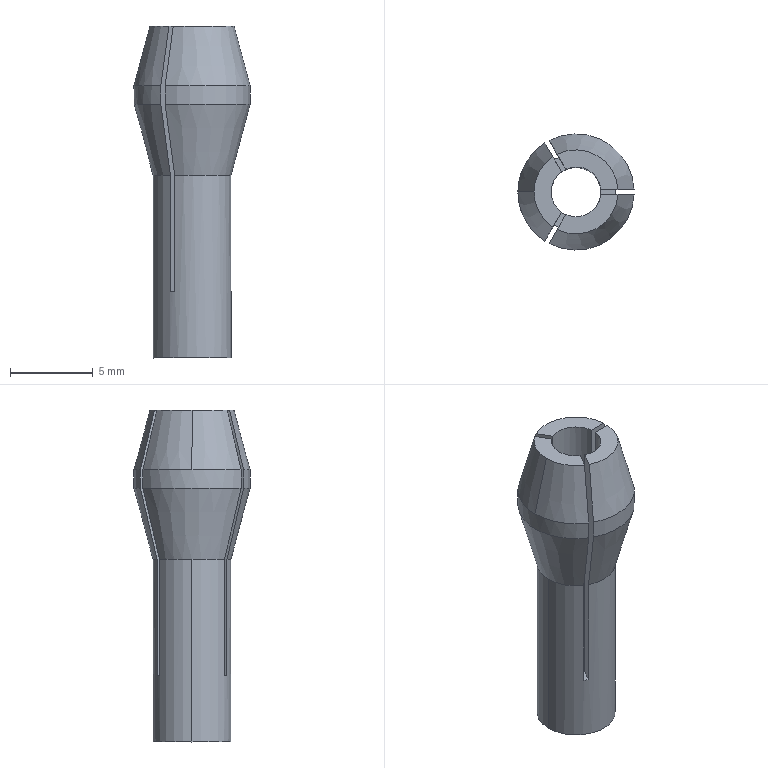Part | SolidWorks | features BaseBody 1 | 1 solid | 27 faces | box 6.997 x 7 x 20 mm | volume 294.902 mm3 | plane 13 | cylinder 7 | cone 7 | commonest cylinder face diameters 7 x3 3 x2 4.7 x2
STEP:
#1=CARTESIAN_POINT('',(482.037,37.715,102.045));
#2=VERTEX_POINT('',#1);
#3=CARTESIAN_POINT('',(479.037,37.715,102.045));
#4=VERTEX_POINT('',#3);
#5=CARTESIAN_POINT('',(480.537,37.715,102.045));
#6=DIRECTION('',(0.000000013,0.,-1.));
#7=DIRECTION('',(1.,0.,0.000000013));
#8=AXIS2_PLACEMENT_3D('',#5,#6,#7);
#9=CIRCLE('',#8,1.5);
#10=EDGE_CURVE('',#2,#4,#9,.T.);
#11=ORIENTED_EDGE('',*,*,#10,.T.);
#12=CARTESIAN_POINT('',(479.037,37.715,122.045));
#13=VERTEX_POINT('',#12);
#14=CARTESIAN_POINT('',(479.037,37.715,102.045));
#15=DIRECTION('',(-0.000000013,0.,1.));
#16=VECTOR('',#15,1000.);
#17=LINE('',#14,#16);
#18=EDGE_CURVE('',#4,#13,#17,.T.);
#19=ORIENTED_EDGE('',*,*,#18,.T.);
#20=CARTESIAN_POINT('',(479.661,36.497,122.045));
#21=VERTEX_POINT('',#20);
#22=CARTESIAN_POINT('',(480.537,37.715,122.045));
#23=DIRECTION('',(-0.000000013,0.,1.));
#24=DIRECTION('',(1.,0.,0.000000013));
#25=AXIS2_PLACEMENT_3D('',#22,#23,#24);
#26=CIRCLE('',#25,1.5);
#27=EDGE_CURVE('',#13,#21,#26,.T.);
#28=ORIENTED_EDGE('',*,*,#27,.T.);
#29=CARTESIAN_POINT('',(479.661,36.497,106.045));
#30=VERTEX_POINT('',#29);
#31=CARTESIAN_POINT('',(479.661,36.497,112.045));
#32=DIRECTION('',(0.000000013,0.,-1.));
#33=VECTOR('',#32,1000.);
#34=LINE('',#31,#33);
#35=EDGE_CURVE('',#21,#30,#34,.T.);
#36=ORIENTED_EDGE('',*,*,#35,.T.);
#37=CARTESIAN_POINT('',(479.921,36.347,106.045));
#38=VERTEX_POINT('',#37);
#39=CARTESIAN_POINT('',(480.537,37.715,106.045));
#40=DIRECTION('',(-0.000000013,0.,1.));
#41=DIRECTION('',(1.,0.,0.000000013));
#42=AXIS2_PLACEMENT_3D('',#39,#40,#41);
#43=CIRCLE('',#42,1.5);
#44=EDGE_CURVE('',#30,#38,#43,.T.);
#45=ORIENTED_EDGE('',*,*,#44,.T.);
#46=CARTESIAN_POINT('',(479.921,36.347,122.045));
#47=VERTEX_POINT('',#46);
#48=CARTESIAN_POINT('',(479.921,36.347,112.045));
#49=DIRECTION('',(-0.000000013,0.,1.));
#50=VECTOR('',#49,1000.);
#51=LINE('',#48,#50);
#52=EDGE_CURVE('',#38,#47,#51,.T.);
#53=ORIENTED_EDGE('',*,*,#52,.T.);
#54=CARTESIAN_POINT('',(482.029,37.565,122.045));
#55=VERTEX_POINT('',#54);
#56=CARTESIAN_POINT('',(480.537,37.715,122.045));
#57=DIRECTION('',(-0.000000013,0.,1.));
#58=DIRECTION('',(1.,0.,0.000000013));
#59=AXIS2_PLACEMENT_3D('',#56,#57,#58);
#60=CIRCLE('',#59,1.5);
#61=EDGE_CURVE('',#47,#55,#60,.T.);
#62=ORIENTED_EDGE('',*,*,#61,.T.);
#63=CARTESIAN_POINT('',(482.029,37.565,106.045));
#64=VERTEX_POINT('',#63);
#65=CARTESIAN_POINT('',(482.029,37.565,112.045));
#66=DIRECTION('',(0.000000013,0.,-1.));
#67=VECTOR('',#66,1000.);
#68=LINE('',#65,#67);
#69=EDGE_CURVE('',#55,#64,#68,.T.);
#70=ORIENTED_EDGE('',*,*,#69,.T.);
#71=CARTESIAN_POINT('',(482.037,37.715,106.045));
#72=VERTEX_POINT('',#71);
#73=CARTESIAN_POINT('',(480.537,37.715,106.045));
#74=DIRECTION('',(-0.000000013,0.,1.));
#75=DIRECTION('',(1.,0.,0.000000013));
#76=AXIS2_PLACEMENT_3D('',#73,#74,#75);
#77=CIRCLE('',#76,1.5);
#78=EDGE_CURVE('',#64,#72,#77,.T.);
#79=ORIENTED_EDGE('',*,*,#78,.T.);
#80=CARTESIAN_POINT('',(482.037,37.715,102.045));
#81=DIRECTION('',(-0.000000013,0.,1.));
#82=VECTOR('',#81,1000.);
#83=LINE('',#80,#82);
#84=EDGE_CURVE('',#2,#72,#83,.T.);
#85=ORIENTED_EDGE('',*,*,#84,.F.);
#86=EDGE_LOOP('',(#11,#19,#28,#36,#45,#53,#62,#70,#79,#85));
#87=FACE_OUTER_BOUND('',#86,.T.);
#88=CARTESIAN_POINT('',(480.537,37.715,102.045));
#89=DIRECTION('',(-0.000000013,0.,1.));
#90=DIRECTION('',(1.,0.,0.000000013));
#91=AXIS2_PLACEMENT_3D('',#88,#89,#90);
#92=CYLINDRICAL_SURFACE('',#91,1.5);
#93=ADVANCED_FACE('',(#87),#92,.F.);
#94=CARTESIAN_POINT('',(482.887,37.715,102.045));
#95=VERTEX_POINT('',#94);
#96=CARTESIAN_POINT('',(478.187,37.715,102.045));
#97=VERTEX_POINT('',#96);
#98=CARTESIAN_POINT('',(480.537,37.715,102.045));
#99=DIRECTION('',(-0.000000013,0.,1.));
#100=DIRECTION('',(1.,0.,0.000000013));
#101=AXIS2_PLACEMENT_3D('',#98,#99,#100);
#102=CIRCLE('',#101,2.35);
#103=EDGE_CURVE('',#95,#97,#102,.T.);
#104=ORIENTED_EDGE('',*,*,#103,.T.);
#105=CARTESIAN_POINT('',(478.187,37.715,113.045));
#106=VERTEX_POINT('',#105);
#107=CARTESIAN_POINT('',(478.187,37.715,102.045));
#108=DIRECTION('',(-0.000000013,0.,1.));
#109=VECTOR('',#108,1000.);
#110=LINE('',#107,#109);
#111=EDGE_CURVE('',#97,#106,#110,.T.);
#112=ORIENTED_EDGE('',*,*,#111,.T.);
#113=CARTESIAN_POINT('',(479.234,39.671,113.045));
#114=VERTEX_POINT('',#113);
#115=CARTESIAN_POINT('',(480.537,37.715,113.045));
#116=DIRECTION('',(-0.000000013,0.,1.));
#117=DIRECTION('',(0.,1.,0.));
#118=AXIS2_PLACEMENT_3D('',#115,#116,#117);
#119=CIRCLE('',#118,2.35);
#120=EDGE_CURVE('',#114,#106,#119,.T.);
#121=ORIENTED_EDGE('',*,*,#120,.F.);
#122=CARTESIAN_POINT('',(479.234,39.671,106.045));
#123=VERTEX_POINT('',#122);
#124=CARTESIAN_POINT('',(479.234,39.671,107.545));
#125=DIRECTION('',(-0.000000013,0.,1.));
#126=VECTOR('',#125,1000.);
#127=LINE('',#124,#126);
#128=EDGE_CURVE('',#123,#114,#127,.T.);
#129=ORIENTED_EDGE('',*,*,#128,.F.);
#130=CARTESIAN_POINT('',(479.494,39.821,106.045));
#131=VERTEX_POINT('',#130);
#132=CARTESIAN_POINT('',(480.537,37.715,106.045));
#133=DIRECTION('',(-0.000000013,0.,1.));
#134=DIRECTION('',(1.,0.,0.000000013));
#135=AXIS2_PLACEMENT_3D('',#132,#133,#134);
#136=CIRCLE('',#135,2.35);
#137=EDGE_CURVE('',#131,#123,#136,.T.);
#138=ORIENTED_EDGE('',*,*,#137,.F.);
#139=CARTESIAN_POINT('',(479.494,39.821,113.045));
#140=VERTEX_POINT('',#139);
#141=CARTESIAN_POINT('',(479.494,39.821,107.545));
#142=DIRECTION('',(0.000000013,0.,-1.));
#143=VECTOR('',#142,1000.);
#144=LINE('',#141,#143);
#145=EDGE_CURVE('',#140,#131,#144,.T.);
#146=ORIENTED_EDGE('',*,*,#145,.F.);
#147=CARTESIAN_POINT('',(482.882,37.865,113.045));
#148=VERTEX_POINT('',#147);
#149=CARTESIAN_POINT('',(480.537,37.715,113.045));
#150=DIRECTION('',(-0.000000013,0.,1.));
#151=DIRECTION('',(0.,1.,0.));
#152=AXIS2_PLACEMENT_3D('',#149,#150,#151);
#153=CIRCLE('',#152,2.35);
#154=EDGE_CURVE('',#148,#140,#153,.T.);
#155=ORIENTED_EDGE('',*,*,#154,.F.);
#156=CARTESIAN_POINT('',(482.882,37.865,106.045));
#157=VERTEX_POINT('',#156);
#158=CARTESIAN_POINT('',(482.882,37.865,114.045));
#159=DIRECTION('',(0.000000013,0.,-1.));
#160=VECTOR('',#159,1000.);
#161=LINE('',#158,#160);
#162=EDGE_CURVE('',#148,#157,#161,.T.);
#163=ORIENTED_EDGE('',*,*,#162,.T.);
#164=CARTESIAN_POINT('',(482.887,37.715,106.045));
#165=VERTEX_POINT('',#164);
#166=CARTESIAN_POINT('',(480.537,37.715,106.045));
#167=DIRECTION('',(-0.000000013,0.,1.));
#168=DIRECTION('',(1.,0.,0.000000013));
#169=AXIS2_PLACEMENT_3D('',#166,#167,#168);
#170=CIRCLE('',#169,2.35);
#171=EDGE_CURVE('',#165,#157,#170,.T.);
#172=ORIENTED_EDGE('',*,*,#171,.F.);
#173=CARTESIAN_POINT('',(482.887,37.715,102.045));
#174=DIRECTION('',(-0.000000013,0.,1.));
#175=VECTOR('',#174,1000.);
#176=LINE('',#173,#175);
#177=EDGE_CURVE('',#95,#165,#176,.T.);
#178=ORIENTED_EDGE('',*,*,#177,.F.);
#179=EDGE_LOOP('',(#104,#112,#121,#129,#138,#146,#155,#163,#172,#178));
#180=FACE_OUTER_BOUND('',#179,.T.);
#181=CARTESIAN_POINT('',(480.537,37.715,102.045));
#182=DIRECTION('',(-0.000000013,0.,1.));
#183=DIRECTION('',(1.,0.,0.000000013));
#184=AXIS2_PLACEMENT_3D('',#181,#182,#183);
#185=CYLINDRICAL_SURFACE('',#184,2.35);
#186=ADVANCED_FACE('',(#180),#185,.T.);
#187=CARTESIAN_POINT('',(478.004,37.715,122.045));
#188=VERTEX_POINT('',#187);
#189=CARTESIAN_POINT('',(479.143,35.6,122.045));
#190=VERTEX_POINT('',#189);
#191=CARTESIAN_POINT('',(480.537,37.715,122.045));
#192=DIRECTION('',(-0.000000013,0.,1.));
#193=DIRECTION('',(-1.,0.,-0.000000013));
#194=AXIS2_PLACEMENT_3D('',#191,#192,#193);
#195=CIRCLE('',#194,2.533);
#196=EDGE_CURVE('',#188,#190,#195,.T.);
#197=ORIENTED_EDGE('',*,*,#196,.F.);
#198=CARTESIAN_POINT('',(477.037,37.715,118.437));
#199=VERTEX_POINT('',#198);
#200=CARTESIAN_POINT('',(477.037,37.715,118.437));
#201=DIRECTION('',(-0.2588,0.,-0.9659));
#202=VECTOR('',#201,1000.);
#203=LINE('',#200,#202);
#204=EDGE_CURVE('',#188,#199,#203,.T.);
#205=ORIENTED_EDGE('',*,*,#204,.T.);
#206=CARTESIAN_POINT('',(478.659,34.761,118.437));
#207=VERTEX_POINT('',#206);
#208=CARTESIAN_POINT('',(480.537,37.715,118.437));
#209=DIRECTION('',(0.000000013,0.,-1.));
#210=DIRECTION('',(0.,1.,0.));
#211=AXIS2_PLACEMENT_3D('',#208,#209,#210);
#212=CIRCLE('',#211,3.5);
#213=EDGE_CURVE('',#207,#199,#212,.T.);
#214=ORIENTED_EDGE('',*,*,#213,.F.);
#215=CARTESIAN_POINT('',(478.659,34.761,118.437));
#216=CARTESIAN_POINT('',(478.82,35.041,119.64));
#217=CARTESIAN_POINT('',(478.981,35.32,120.842));
#218=CARTESIAN_POINT('',(479.143,35.6,122.045));
#219=B_SPLINE_CURVE_WITH_KNOTS('',3,(#215,#216,#217,#218),.UNSPECIFIED.,.F.,.F.,(4,4),(0.,0.003736),.UNSPECIFIED.);
#220=EDGE_CURVE('',#207,#190,#219,.T.);
#221=ORIENTED_EDGE('',*,*,#220,.T.);
#222=EDGE_LOOP('',(#197,#205,#214,#221));
#223=FACE_OUTER_BOUND('',#222,.T.);
#224=CARTESIAN_POINT('',(480.537,37.715,118.437));
#225=DIRECTION('',(0.000000013,0.,-1.));
#226=DIRECTION('',(-1.,0.,-0.000000013));
#227=AXIS2_PLACEMENT_3D('',#224,#225,#226);
#228=CONICAL_SURFACE('',#227,3.5,0.2618);
#229=ADVANCED_FACE('',(#223),#228,.T.);
#230=ORIENTED_EDGE('',*,*,#18,.F.);
#231=CARTESIAN_POINT('',(480.537,37.715,102.045));
#232=DIRECTION('',(0.000000013,0.,-1.));
#233=DIRECTION('',(1.,0.,0.000000013));
#234=AXIS2_PLACEMENT_3D('',#231,#232,#233);
#235=CIRCLE('',#234,1.5);
#236=EDGE_CURVE('',#4,#2,#235,.T.);
#237=ORIENTED_EDGE('',*,*,#236,.T.);
#238=ORIENTED_EDGE('',*,*,#84,.T.);
#239=CARTESIAN_POINT('',(482.029,37.865,106.045));
#240=VERTEX_POINT('',#239);
#241=CARTESIAN_POINT('',(480.537,37.715,106.045));
#242=DIRECTION('',(-0.000000013,0.,1.));
#243=DIRECTION('',(1.,0.,0.000000013));
#244=AXIS2_PLACEMENT_3D('',#241,#242,#243);
#245=CIRCLE('',#244,1.5);
#246=EDGE_CURVE('',#72,#240,#245,.T.);
#247=ORIENTED_EDGE('',*,*,#246,.T.);
#248=CARTESIAN_POINT('',(482.029,37.865,122.045));
#249=VERTEX_POINT('',#248);
#250=CARTESIAN_POINT('',(482.029,37.865,112.045));
#251=DIRECTION('',(-0.000000013,0.,1.));
#252=VECTOR('',#251,1000.);
#253=LINE('',#250,#252);
#254=EDGE_CURVE('',#240,#249,#253,.T.);
#255=ORIENTED_EDGE('',*,*,#254,.T.);
#256=CARTESIAN_POINT('',(479.921,39.082,122.045));
#257=VERTEX_POINT('',#256);
#258=CARTESIAN_POINT('',(480.537,37.715,122.045));
#259=DIRECTION('',(-0.000000013,0.,1.));
#260=DIRECTION('',(1.,0.,0.000000013));
#261=AXIS2_PLACEMENT_3D('',#258,#259,#260);
#262=CIRCLE('',#261,1.5);
#263=EDGE_CURVE('',#249,#257,#262,.T.);
#264=ORIENTED_EDGE('',*,*,#263,.T.);
#265=CARTESIAN_POINT('',(479.921,39.082,106.045));
#266=VERTEX_POINT('',#265);
#267=CARTESIAN_POINT('',(479.921,39.082,112.045));
#268=DIRECTION('',(0.000000013,0.,-1.));
#269=VECTOR('',#268,1000.);
#270=LINE('',#267,#269);
#271=EDGE_CURVE('',#257,#266,#270,.T.);
#272=ORIENTED_EDGE('',*,*,#271,.T.);
#273=CARTESIAN_POINT('',(479.661,38.932,106.045));
#274=VERTEX_POINT('',#273);
#275=CARTESIAN_POINT('',(480.537,37.715,106.045));
#276=DIRECTION('',(-0.000000013,0.,1.));
#277=DIRECTION('',(1.,0.,0.000000013));
#278=AXIS2_PLACEMENT_3D('',#275,#276,#277);
#279=CIRCLE('',#278,1.5);
#280=EDGE_CURVE('',#266,#274,#279,.T.);
#281=ORIENTED_EDGE('',*,*,#280,.T.);
#282=CARTESIAN_POINT('',(479.661,38.932,122.045));
#283=VERTEX_POINT('',#282);
#284=CARTESIAN_POINT('',(479.661,38.932,112.045));
#285=DIRECTION('',(-0.000000013,0.,1.));
#286=VECTOR('',#285,1000.);
#287=LINE('',#284,#286);
#288=EDGE_CURVE('',#274,#283,#287,.T.);
#289=ORIENTED_EDGE('',*,*,#288,.T.);
#290=CARTESIAN_POINT('',(480.537,37.715,122.045));
#291=DIRECTION('',(-0.000000013,0.,1.));
#292=DIRECTION('',(1.,0.,0.000000013));
#293=AXIS2_PLACEMENT_3D('',#290,#291,#292);
#294=CIRCLE('',#293,1.5);
#295=EDGE_CURVE('',#283,#13,#294,.T.);
#296=ORIENTED_EDGE('',*,*,#295,.T.);
#297=EDGE_LOOP('',(#230,#237,#238,#247,#255,#264,#272,#281,#289,#296));
#298=FACE_OUTER_BOUND('',#297,.T.);
#299=CARTESIAN_POINT('',(480.537,37.715,102.045));
#300=DIRECTION('',(-0.000000013,0.,1.));
#301=DIRECTION('',(1.,0.,0.000000013));
#302=AXIS2_PLACEMENT_3D('',#299,#300,#301);
#303=CYLINDRICAL_SURFACE('',#302,1.5);
#304=ADVANCED_FACE('',(#298),#303,.F.);
#305=ORIENTED_EDGE('',*,*,#10,.F.);
#306=ORIENTED_EDGE('',*,*,#236,.F.);
#307=EDGE_LOOP('',(#305,#306));
#308=FACE_BOUND('',#307,.T.);
#309=ORIENTED_EDGE('',*,*,#103,.F.);
#310=CARTESIAN_POINT('',(480.537,37.715,102.045));
#311=DIRECTION('',(-0.000000013,0.,1.));
#312=DIRECTION('',(1.,0.,0.000000013));
#313=AXIS2_PLACEMENT_3D('',#310,#311,#312);
#314=CIRCLE('',#313,2.35);
#315=EDGE_CURVE('',#97,#95,#314,.T.);
#316=ORIENTED_EDGE('',*,*,#315,.F.);
#317=EDGE_LOOP('',(#309,#316));
#318=FACE_OUTER_BOUND('',#317,.T.);
#319=CARTESIAN_POINT('',(482.981,35.271,102.045));
#320=DIRECTION('',(-0.000000013,0.,1.));
#321=DIRECTION('',(0.,1.,0.));
#322=AXIS2_PLACEMENT_3D('',#319,#320,#321);
#323=PLANE('',#322);
#324=ADVANCED_FACE('',(#308,#318),#323,.F.);
#325=CARTESIAN_POINT('',(483.066,37.865,122.045));
#326=VERTEX_POINT('',#325);
#327=CARTESIAN_POINT('',(479.402,39.98,122.045));
#328=VERTEX_POINT('',#327);
#329=CARTESIAN_POINT('',(480.537,37.715,122.045));
#330=DIRECTION('',(-0.000000013,0.,1.));
#331=DIRECTION('',(-1.,0.,-0.000000013));
#332=AXIS2_PLACEMENT_3D('',#329,#330,#331);
#333=CIRCLE('',#332,2.533);
#334=EDGE_CURVE('',#326,#328,#333,.T.);
#335=ORIENTED_EDGE('',*,*,#334,.T.);
#336=CARTESIAN_POINT('',(479.402,39.98,122.045));
#337=DIRECTION('',(0.5,-0.866,0.000000006));
#338=VECTOR('',#337,1000.);
#339=LINE('',#336,#338);
#340=EDGE_CURVE('',#328,#257,#339,.T.);
#341=ORIENTED_EDGE('',*,*,#340,.T.);
#342=ORIENTED_EDGE('',*,*,#263,.F.);
#343=CARTESIAN_POINT('',(480.535,37.865,122.045));
#344=DIRECTION('',(1.,0.,0.000000013));
#345=VECTOR('',#344,1000.);
#346=LINE('',#343,#345);
#347=EDGE_CURVE('',#249,#326,#346,.T.);
#348=ORIENTED_EDGE('',*,*,#347,.T.);
#349=EDGE_LOOP('',(#335,#341,#342,#348));
#350=FACE_OUTER_BOUND('',#349,.T.);
#351=CARTESIAN_POINT('',(483.167,35.078,122.045));
#352=DIRECTION('',(-0.000000013,0.,1.));
#353=DIRECTION('',(0.,1.,0.));
#354=AXIS2_PLACEMENT_3D('',#351,#352,#353);
#355=PLANE('',#354);
#356=ADVANCED_FACE('',(#350),#355,.T.);
#357=ORIENTED_EDGE('',*,*,#254,.F.);
#358=CARTESIAN_POINT('',(483.031,37.865,106.045));
#359=DIRECTION('',(-1.,0.,-0.000000013));
#360=VECTOR('',#359,1000.);
#361=LINE('',#358,#360);
#362=EDGE_CURVE('',#157,#240,#361,.T.);
#363=ORIENTED_EDGE('',*,*,#362,.F.);
#364=ORIENTED_EDGE('',*,*,#162,.F.);
#365=CARTESIAN_POINT('',(484.034,37.865,117.337));
#366=VERTEX_POINT('',#365);
#367=CARTESIAN_POINT('',(484.034,37.865,117.337));
#368=CARTESIAN_POINT('',(483.65,37.865,115.906));
#369=CARTESIAN_POINT('',(483.266,37.865,114.476));
#370=CARTESIAN_POINT('',(482.882,37.865,113.045));
#371=B_SPLINE_CURVE_WITH_KNOTS('',3,(#367,#368,#369,#370),.UNSPECIFIED.,.F.,.F.,(4,4),(0.,0.004444),.UNSPECIFIED.);
#372=EDGE_CURVE('',#366,#148,#371,.T.);
#373=ORIENTED_EDGE('',*,*,#372,.F.);
#374=CARTESIAN_POINT('',(484.034,37.865,118.437));
#375=VERTEX_POINT('',#374);
#376=CARTESIAN_POINT('',(484.034,37.865,117.887));
#377=DIRECTION('',(-0.000000013,0.,1.));
#378=VECTOR('',#377,1000.);
#379=LINE('',#376,#378);
#380=EDGE_CURVE('',#366,#375,#379,.T.);
#381=ORIENTED_EDGE('',*,*,#380,.T.);
#382=CARTESIAN_POINT('',(483.066,37.865,122.045));
#383=CARTESIAN_POINT('',(483.388,37.865,120.842));
#384=CARTESIAN_POINT('',(483.711,37.865,119.64));
#385=CARTESIAN_POINT('',(484.034,37.865,118.437));
#386=B_SPLINE_CURVE_WITH_KNOTS('',3,(#382,#383,#384,#385),.UNSPECIFIED.,.F.,.F.,(4,4),(0.,0.003736),.UNSPECIFIED.);
#387=EDGE_CURVE('',#326,#375,#386,.T.);
#388=ORIENTED_EDGE('',*,*,#387,.F.);
#389=ORIENTED_EDGE('',*,*,#347,.F.);
#390=EDGE_LOOP('',(#357,#363,#364,#373,#381,#388,#389));
#391=FACE_OUTER_BOUND('',#390,.T.);
#392=CARTESIAN_POINT('',(484.074,37.865,105.725));
#393=DIRECTION('',(0.,1.,0.));
#394=DIRECTION('',(-1.,0.,-0.000000013));
#395=AXIS2_PLACEMENT_3D('',#392,#393,#394);
#396=PLANE('',#395);
#397=ADVANCED_FACE('',(#391),#396,.F.);
#398=ORIENTED_EDGE('',*,*,#78,.F.);
#399=CARTESIAN_POINT('',(482.882,37.565,106.045));
#400=VERTEX_POINT('',#399);
#401=CARTESIAN_POINT('',(482.458,37.565,106.045));
#402=DIRECTION('',(1.,0.,0.000000013));
#403=VECTOR('',#402,1000.);
#404=LINE('',#401,#403);
#405=EDGE_CURVE('',#64,#400,#404,.T.);
#406=ORIENTED_EDGE('',*,*,#405,.T.);
#407=CARTESIAN_POINT('',(480.537,37.715,106.045));
#408=DIRECTION('',(-0.000000013,0.,1.));
#409=DIRECTION('',(1.,0.,0.000000013));
#410=AXIS2_PLACEMENT_3D('',#407,#408,#409);
#411=CIRCLE('',#410,2.35);
#412=EDGE_CURVE('',#400,#165,#411,.T.);
#413=ORIENTED_EDGE('',*,*,#412,.T.);
#414=ORIENTED_EDGE('',*,*,#171,.T.);
#415=ORIENTED_EDGE('',*,*,#362,.T.);
#416=ORIENTED_EDGE('',*,*,#246,.F.);
#417=EDGE_LOOP('',(#398,#406,#413,#414,#415,#416));
#418=FACE_OUTER_BOUND('',#417,.T.);
#419=CARTESIAN_POINT('',(482.003,37.891,106.045));
#420=DIRECTION('',(-0.000000013,0.,1.));
#421=DIRECTION('',(0.,-1.,0.));
#422=AXIS2_PLACEMENT_3D('',#419,#420,#421);
#423=PLANE('',#422);
#424=ADVANCED_FACE('',(#418),#423,.T.);
#425=CARTESIAN_POINT('',(484.034,37.565,118.437));
#426=VERTEX_POINT('',#425);
#427=CARTESIAN_POINT('',(483.066,37.565,122.045));
#428=VERTEX_POINT('',#427);
#429=CARTESIAN_POINT('',(484.034,37.565,118.437));
#430=CARTESIAN_POINT('',(483.711,37.565,119.64));
#431=CARTESIAN_POINT('',(483.388,37.565,120.842));
#432=CARTESIAN_POINT('',(483.066,37.565,122.045));
#433=B_SPLINE_CURVE_WITH_KNOTS('',3,(#429,#430,#431,#432),.UNSPECIFIED.,.F.,.F.,(4,4),(0.,0.003736),.UNSPECIFIED.);
#434=EDGE_CURVE('',#426,#428,#433,.T.);
#435=ORIENTED_EDGE('',*,*,#434,.F.);
#436=CARTESIAN_POINT('',(484.034,37.565,117.337));
#437=VERTEX_POINT('',#436);
#438=CARTESIAN_POINT('',(484.034,37.565,117.887));
#439=DIRECTION('',(0.000000013,0.,-1.));
#440=VECTOR('',#439,1000.);
#441=LINE('',#438,#440);
#442=EDGE_CURVE('',#426,#437,#441,.T.);
#443=ORIENTED_EDGE('',*,*,#442,.T.);
#444=CARTESIAN_POINT('',(482.882,37.565,113.045));
#445=VERTEX_POINT('',#444);
#446=CARTESIAN_POINT('',(482.882,37.565,113.045));
#447=CARTESIAN_POINT('',(483.205,37.565,114.247));
#448=CARTESIAN_POINT('',(483.527,37.565,115.449));
#449=CARTESIAN_POINT('',(483.85,37.565,116.651));
#450=CARTESIAN_POINT('',(483.911,37.565,116.88));
#451=CARTESIAN_POINT('',(483.972,37.565,117.108));
#452=CARTESIAN_POINT('',(484.034,37.565,117.337));
#453=B_SPLINE_CURVE_WITH_KNOTS('',3,(#446,#447,#448,#449,#450,#451,#452),.UNSPECIFIED.,.F.,.F.,(4,3,4),(0.,0.003734,0.004444),.UNSPECIFIED.);
#454=EDGE_CURVE('',#445,#437,#453,.T.);
#455=ORIENTED_EDGE('',*,*,#454,.F.);
#456=CARTESIAN_POINT('',(482.882,37.565,114.045));
#457=DIRECTION('',(-0.000000013,0.,1.));
#458=VECTOR('',#457,1000.);
#459=LINE('',#456,#458);
#460=EDGE_CURVE('',#400,#445,#459,.T.);
#461=ORIENTED_EDGE('',*,*,#460,.F.);
#462=ORIENTED_EDGE('',*,*,#405,.F.);
#463=ORIENTED_EDGE('',*,*,#69,.F.);
#464=CARTESIAN_POINT('',(483.031,37.565,122.045));
#465=DIRECTION('',(-1.,0.,-0.000000013));
#466=VECTOR('',#465,1000.);
#467=LINE('',#464,#466);
#468=EDGE_CURVE('',#428,#55,#467,.T.);
#469=ORIENTED_EDGE('',*,*,#468,.F.);
#470=EDGE_LOOP('',(#435,#443,#455,#461,#462,#463,#469));
#471=FACE_OUTER_BOUND('',#470,.T.);
#472=CARTESIAN_POINT('',(481.989,37.565,105.725));
#473=DIRECTION('',(0.,-1.,0.));
#474=DIRECTION('',(1.,0.,0.000000013));
#475=AXIS2_PLACEMENT_3D('',#472,#473,#474);
#476=PLANE('',#475);
#477=ADVANCED_FACE('',(#471),#476,.F.);
#478=ORIENTED_EDGE('',*,*,#61,.F.);
#479=CARTESIAN_POINT('',(479.402,35.45,122.045));
#480=VERTEX_POINT('',#479);
#481=CARTESIAN_POINT('',(479.921,36.347,122.045));
#482=DIRECTION('',(-0.5,-0.866,-0.000000006));
#483=VECTOR('',#482,1000.);
#484=LINE('',#481,#483);
#485=EDGE_CURVE('',#47,#480,#484,.T.);
#486=ORIENTED_EDGE('',*,*,#485,.T.);
#487=CARTESIAN_POINT('',(480.537,37.715,122.045));
#488=DIRECTION('',(-0.000000013,0.,1.));
#489=DIRECTION('',(-1.,0.,-0.000000013));
#490=AXIS2_PLACEMENT_3D('',#487,#488,#489);
#491=CIRCLE('',#490,2.533);
#492=EDGE_CURVE('',#480,#428,#491,.T.);
#493=ORIENTED_EDGE('',*,*,#492,.T.);
#494=ORIENTED_EDGE('',*,*,#468,.T.);
#495=EDGE_LOOP('',(#478,#486,#493,#494));
#496=FACE_OUTER_BOUND('',#495,.T.);
#497=CARTESIAN_POINT('',(483.167,35.078,122.045));
#498=DIRECTION('',(-0.000000013,0.,1.));
#499=DIRECTION('',(0.,1.,0.));
#500=AXIS2_PLACEMENT_3D('',#497,#498,#499);
#501=PLANE('',#500);
#502=ADVANCED_FACE('',(#496),#501,.T.);
#503=ORIENTED_EDGE('',*,*,#111,.F.);
#504=ORIENTED_EDGE('',*,*,#315,.T.);
#505=ORIENTED_EDGE('',*,*,#177,.T.);
#506=ORIENTED_EDGE('',*,*,#412,.F.);
#507=ORIENTED_EDGE('',*,*,#460,.T.);
#508=CARTESIAN_POINT('',(479.494,35.609,113.045));
#509=VERTEX_POINT('',#508);
#510=CARTESIAN_POINT('',(480.537,37.715,113.045));
#511=DIRECTION('',(-0.000000013,0.,1.));
#512=DIRECTION('',(0.,1.,0.));
#513=AXIS2_PLACEMENT_3D('',#510,#511,#512);
#514=CIRCLE('',#513,2.35);
#515=EDGE_CURVE('',#509,#445,#514,.T.);
#516=ORIENTED_EDGE('',*,*,#515,.F.);
#517=CARTESIAN_POINT('',(479.494,35.609,106.045));
#518=VERTEX_POINT('',#517);
#519=CARTESIAN_POINT('',(479.494,35.609,107.545));
#520=DIRECTION('',(-0.000000013,0.,1.));
#521=VECTOR('',#520,1000.);
#522=LINE('',#519,#521);
#523=EDGE_CURVE('',#518,#509,#522,.T.);
#524=ORIENTED_EDGE('',*,*,#523,.F.);
#525=CARTESIAN_POINT('',(479.234,35.759,106.045));
#526=VERTEX_POINT('',#525);
#527=CARTESIAN_POINT('',(480.537,37.715,106.045));
#528=DIRECTION('',(-0.000000013,0.,1.));
#529=DIRECTION('',(1.,0.,0.000000013));
#530=AXIS2_PLACEMENT_3D('',#527,#528,#529);
#531=CIRCLE('',#530,2.35);
#532=EDGE_CURVE('',#526,#518,#531,.T.);
#533=ORIENTED_EDGE('',*,*,#532,.F.);
#534=CARTESIAN_POINT('',(479.234,35.759,113.045));
#535=VERTEX_POINT('',#534);
#536=CARTESIAN_POINT('',(479.234,35.759,107.545));
#537=DIRECTION('',(0.000000013,0.,-1.));
#538=VECTOR('',#537,1000.);
#539=LINE('',#536,#538);
#540=EDGE_CURVE('',#535,#526,#539,.T.);
#541=ORIENTED_EDGE('',*,*,#540,.F.);
#542=CARTESIAN_POINT('',(480.537,37.715,113.045));
#543=DIRECTION('',(-0.000000013,0.,1.));
#544=DIRECTION('',(0.,1.,0.));
#545=AXIS2_PLACEMENT_3D('',#542,#543,#544);
#546=CIRCLE('',#545,2.35);
#547=EDGE_CURVE('',#106,#535,#546,.T.);
#548=ORIENTED_EDGE('',*,*,#547,.F.);
#549=EDGE_LOOP('',(#503,#504,#505,#506,#507,#516,#524,#533,#541,#548));
#550=FACE_OUTER_BOUND('',#549,.T.);
#551=CARTESIAN_POINT('',(480.537,37.715,102.045));
#552=DIRECTION('',(-0.000000013,0.,1.));
#553=DIRECTION('',(1.,0.,0.000000013));
#554=AXIS2_PLACEMENT_3D('',#551,#552,#553);
#555=CYLINDRICAL_SURFACE('',#554,2.35);
#556=ADVANCED_FACE('',(#550),#555,.T.);
#557=ORIENTED_EDGE('',*,*,#52,.F.);
#558=CARTESIAN_POINT('',(479.419,35.479,106.045));
#559=DIRECTION('',(0.5,0.866,0.000000006));
#560=VECTOR('',#559,1000.);
#561=LINE('',#558,#560);
#562=EDGE_CURVE('',#518,#38,#561,.T.);
#563=ORIENTED_EDGE('',*,*,#562,.F.);
#564=ORIENTED_EDGE('',*,*,#523,.T.);
#565=CARTESIAN_POINT('',(478.918,34.611,117.337));
#566=VERTEX_POINT('',#565);
#567=CARTESIAN_POINT('',(478.918,34.611,117.337));
#568=CARTESIAN_POINT('',(479.11,34.944,115.906));
#569=CARTESIAN_POINT('',(479.302,35.276,114.476));
#570=CARTESIAN_POINT('',(479.494,35.609,113.045));
#571=B_SPLINE_CURVE_WITH_KNOTS('',3,(#567,#568,#569,#570),.UNSPECIFIED.,.F.,.F.,(4,4),(0.,0.004444),.UNSPECIFIED.);
#572=EDGE_CURVE('',#566,#509,#571,.T.);
#573=ORIENTED_EDGE('',*,*,#572,.F.);
#574=CARTESIAN_POINT('',(478.918,34.611,118.437));
#575=VERTEX_POINT('',#574);
#576=CARTESIAN_POINT('',(478.918,34.611,114.045));
#577=DIRECTION('',(0.000000013,0.,-1.));
#578=VECTOR('',#577,1000.);
#579=LINE('',#576,#578);
#580=EDGE_CURVE('',#575,#566,#579,.T.);
#581=ORIENTED_EDGE('',*,*,#580,.F.);
#582=CARTESIAN_POINT('',(479.402,35.45,122.045));
#583=CARTESIAN_POINT('',(479.241,35.17,120.842));
#584=CARTESIAN_POINT('',(479.08,34.891,119.64));
#585=CARTESIAN_POINT('',(478.918,34.611,118.437));
#586=B_SPLINE_CURVE_WITH_KNOTS('',3,(#582,#583,#584,#585),.UNSPECIFIED.,.F.,.F.,(4,4),(0.,0.003736),.UNSPECIFIED.);
#587=EDGE_CURVE('',#480,#575,#586,.T.);
#588=ORIENTED_EDGE('',*,*,#587,.F.);
#589=ORIENTED_EDGE('',*,*,#485,.F.);
#590=EDGE_LOOP('',(#557,#563,#564,#573,#581,#588,#589));
#591=FACE_OUTER_BOUND('',#590,.T.);
#592=CARTESIAN_POINT('',(478.898,34.577,105.725));
#593=DIRECTION('',(0.866,-0.5,0.000000011));
#594=DIRECTION('',(0.5,0.866,0.000000006));
#595=AXIS2_PLACEMENT_3D('',#592,#593,#594);
#596=PLANE('',#595);
#597=ADVANCED_FACE('',(#591),#596,.F.);
#598=ORIENTED_EDGE('',*,*,#44,.F.);
#599=CARTESIAN_POINT('',(479.446,36.126,106.045));
#600=DIRECTION('',(-0.5,-0.866,-0.000000006));
#601=VECTOR('',#600,1000.);
#602=LINE('',#599,#601);
#603=EDGE_CURVE('',#30,#526,#602,.T.);
#604=ORIENTED_EDGE('',*,*,#603,.T.);
#605=ORIENTED_EDGE('',*,*,#532,.T.);
#606=ORIENTED_EDGE('',*,*,#562,.T.);
#607=EDGE_LOOP('',(#598,#604,#605,#606));
#608=FACE_OUTER_BOUND('',#607,.T.);
#609=CARTESIAN_POINT('',(479.957,36.357,106.045));
#610=DIRECTION('',(-0.000000013,0.,1.));
#611=DIRECTION('',(-0.866,0.5,-0.000000011));
#612=AXIS2_PLACEMENT_3D('',#609,#610,#611);
#613=PLANE('',#612);
#614=ADVANCED_FACE('',(#608),#613,.T.);
#615=ORIENTED_EDGE('',*,*,#220,.F.);
#616=CARTESIAN_POINT('',(478.659,34.761,117.337));
#617=VERTEX_POINT('',#616);
#618=CARTESIAN_POINT('',(478.659,34.761,117.887));
#619=DIRECTION('',(0.000000013,0.,-1.));
#620=VECTOR('',#619,1000.);
#621=LINE('',#618,#620);
#622=EDGE_CURVE('',#207,#617,#621,.T.);
#623=ORIENTED_EDGE('',*,*,#622,.T.);
#624=CARTESIAN_POINT('',(479.234,35.759,113.045));
#625=CARTESIAN_POINT('',(479.073,35.479,114.247));
#626=CARTESIAN_POINT('',(478.912,35.2,115.449));
#627=CARTESIAN_POINT('',(478.751,34.921,116.651));
#628=CARTESIAN_POINT('',(478.72,34.868,116.88));
#629=CARTESIAN_POINT('',(478.689,34.815,117.108));
#630=CARTESIAN_POINT('',(478.659,34.761,117.337));
#631=B_SPLINE_CURVE_WITH_KNOTS('',3,(#624,#625,#626,#627,#628,#629,#630),.UNSPECIFIED.,.F.,.F.,(4,3,4),(0.,0.003734,0.004444),.UNSPECIFIED.);
#632=EDGE_CURVE('',#535,#617,#631,.T.);
#633=ORIENTED_EDGE('',*,*,#632,.F.);
#634=ORIENTED_EDGE('',*,*,#540,.T.);
#635=ORIENTED_EDGE('',*,*,#603,.F.);
#636=ORIENTED_EDGE('',*,*,#35,.F.);
#637=CARTESIAN_POINT('',(479.16,35.629,122.045));
#638=DIRECTION('',(0.5,0.866,0.000000006));
#639=VECTOR('',#638,1000.);
#640=LINE('',#637,#639);
#641=EDGE_CURVE('',#190,#21,#640,.T.);
#642=ORIENTED_EDGE('',*,*,#641,.F.);
#643=EDGE_LOOP('',(#615,#623,#633,#634,#635,#636,#642));
#644=FACE_OUTER_BOUND('',#643,.T.);
#645=CARTESIAN_POINT('',(479.681,36.532,105.725));
#646=DIRECTION('',(-0.866,0.5,-0.000000011));
#647=DIRECTION('',(-0.5,-0.866,-0.000000006));
#648=AXIS2_PLACEMENT_3D('',#645,#646,#647);
#649=PLANE('',#648);
#650=ADVANCED_FACE('',(#644),#649,.F.);
#651=ORIENTED_EDGE('',*,*,#641,.T.);
#652=ORIENTED_EDGE('',*,*,#27,.F.);
#653=ORIENTED_EDGE('',*,*,#295,.F.);
#654=CARTESIAN_POINT('',(479.143,39.83,122.045));
#655=VERTEX_POINT('',#654);
#656=CARTESIAN_POINT('',(479.661,38.932,122.045));
#657=DIRECTION('',(-0.5,0.866,-0.000000006));
#658=VECTOR('',#657,1000.);
#659=LINE('',#656,#658);
#660=EDGE_CURVE('',#283,#655,#659,.T.);
#661=ORIENTED_EDGE('',*,*,#660,.T.);
#662=CARTESIAN_POINT('',(480.537,37.715,122.045));
#663=DIRECTION('',(-0.000000013,0.,1.));
#664=DIRECTION('',(-1.,0.,-0.000000013));
#665=AXIS2_PLACEMENT_3D('',#662,#663,#664);
#666=CIRCLE('',#665,2.533);
#667=EDGE_CURVE('',#655,#188,#666,.T.);
#668=ORIENTED_EDGE('',*,*,#667,.T.);
#669=ORIENTED_EDGE('',*,*,#196,.T.);
#670=EDGE_LOOP('',(#651,#652,#653,#661,#668,#669));
#671=FACE_OUTER_BOUND('',#670,.T.);
#672=CARTESIAN_POINT('',(483.167,35.078,122.045));
#673=DIRECTION('',(-0.000000013,0.,1.));
#674=DIRECTION('',(0.,1.,0.));
#675=AXIS2_PLACEMENT_3D('',#672,#673,#674);
#676=PLANE('',#675);
#677=ADVANCED_FACE('',(#671),#676,.T.);
#678=ORIENTED_EDGE('',*,*,#288,.F.);
#679=CARTESIAN_POINT('',(479.16,39.8,106.045));
#680=DIRECTION('',(0.5,-0.866,0.000000006));
#681=VECTOR('',#680,1000.);
#682=LINE('',#679,#681);
#683=EDGE_CURVE('',#123,#274,#682,.T.);
#684=ORIENTED_EDGE('',*,*,#683,.F.);
#685=ORIENTED_EDGE('',*,*,#128,.T.);
#686=CARTESIAN_POINT('',(478.659,40.668,117.337));
#687=VERTEX_POINT('',#686);
#688=CARTESIAN_POINT('',(478.659,40.668,117.337));
#689=CARTESIAN_POINT('',(478.85,40.336,115.906));
#690=CARTESIAN_POINT('',(479.042,40.003,114.476));
#691=CARTESIAN_POINT('',(479.234,39.671,113.045));
#692=B_SPLINE_CURVE_WITH_KNOTS('',3,(#688,#689,#690,#691),.UNSPECIFIED.,.F.,.F.,(4,4),(0.,0.004444),.UNSPECIFIED.);
#693=EDGE_CURVE('',#687,#114,#692,.T.);
#694=ORIENTED_EDGE('',*,*,#693,.F.);
#695=CARTESIAN_POINT('',(478.659,40.668,118.437));
#696=VERTEX_POINT('',#695);
#697=CARTESIAN_POINT('',(478.659,40.668,117.887));
#698=DIRECTION('',(-0.000000013,0.,1.));
#699=VECTOR('',#698,1000.);
#700=LINE('',#697,#699);
#701=EDGE_CURVE('',#687,#696,#700,.T.);
#702=ORIENTED_EDGE('',*,*,#701,.T.);
#703=CARTESIAN_POINT('',(479.143,39.83,122.045));
#704=CARTESIAN_POINT('',(478.981,40.109,120.842));
#705=CARTESIAN_POINT('',(478.82,40.389,119.64));
#706=CARTESIAN_POINT('',(478.659,40.668,118.437));
#707=B_SPLINE_CURVE_WITH_KNOTS('',3,(#703,#704,#705,#706),.UNSPECIFIED.,.F.,.F.,(4,4),(0.,0.003736),.UNSPECIFIED.);
#708=EDGE_CURVE('',#655,#696,#707,.T.);
#709=ORIENTED_EDGE('',*,*,#708,.F.);
#710=ORIENTED_EDGE('',*,*,#660,.F.);
#711=EDGE_LOOP('',(#678,#684,#685,#694,#702,#709,#710));
#712=FACE_OUTER_BOUND('',#711,.T.);
#713=CARTESIAN_POINT('',(478.639,40.703,105.725));
#714=DIRECTION('',(-0.866,-0.5,-0.000000011));
#715=DIRECTION('',(0.5,-0.866,0.000000006));
#716=AXIS2_PLACEMENT_3D('',#713,#714,#715);
#717=PLANE('',#716);
#718=ADVANCED_FACE('',(#712),#717,.F.);
#719=ORIENTED_EDGE('',*,*,#280,.F.);
#720=CARTESIAN_POINT('',(479.706,39.454,106.045));
#721=DIRECTION('',(-0.5,0.866,-0.000000006));
#722=VECTOR('',#721,1000.);
#723=LINE('',#720,#722);
#724=EDGE_CURVE('',#266,#131,#723,.T.);
#725=ORIENTED_EDGE('',*,*,#724,.T.);
#726=ORIENTED_EDGE('',*,*,#137,.T.);
#727=ORIENTED_EDGE('',*,*,#683,.T.);
#728=EDGE_LOOP('',(#719,#725,#726,#727));
#729=FACE_OUTER_BOUND('',#728,.T.);
#730=CARTESIAN_POINT('',(479.651,38.896,106.045));
#731=DIRECTION('',(-0.000000013,0.,1.));
#732=DIRECTION('',(0.866,0.5,0.000000011));
#733=AXIS2_PLACEMENT_3D('',#730,#731,#732);
#734=PLANE('',#733);
#735=ADVANCED_FACE('',(#729),#734,.T.);
#736=CARTESIAN_POINT('',(478.918,40.818,118.437));
#737=VERTEX_POINT('',#736);
#738=CARTESIAN_POINT('',(478.918,40.818,118.437));
#739=CARTESIAN_POINT('',(479.08,40.539,119.64));
#740=CARTESIAN_POINT('',(479.241,40.259,120.842));
#741=CARTESIAN_POINT('',(479.402,39.98,122.045));
#742=B_SPLINE_CURVE_WITH_KNOTS('',3,(#738,#739,#740,#741),.UNSPECIFIED.,.F.,.F.,(4,4),(0.,0.003736),.UNSPECIFIED.);
#743=EDGE_CURVE('',#737,#328,#742,.T.);
#744=ORIENTED_EDGE('',*,*,#743,.F.);
#745=CARTESIAN_POINT('',(478.918,40.818,117.337));
#746=VERTEX_POINT('',#745);
#747=CARTESIAN_POINT('',(478.918,40.818,114.045));
#748=DIRECTION('',(-0.000000013,0.,1.));
#749=VECTOR('',#748,1000.);
#750=LINE('',#747,#749);
#751=EDGE_CURVE('',#746,#737,#750,.T.);
#752=ORIENTED_EDGE('',*,*,#751,.F.);
#753=CARTESIAN_POINT('',(479.494,39.821,113.045));
#754=CARTESIAN_POINT('',(479.333,40.1,114.247));
#755=CARTESIAN_POINT('',(479.172,40.38,115.449));
#756=CARTESIAN_POINT('',(479.01,40.659,116.651));
#757=CARTESIAN_POINT('',(478.98,40.712,116.88));
#758=CARTESIAN_POINT('',(478.949,40.765,117.108));
#759=CARTESIAN_POINT('',(478.918,40.818,117.337));
#760=B_SPLINE_CURVE_WITH_KNOTS('',3,(#753,#754,#755,#756,#757,#758,#759),.UNSPECIFIED.,.F.,.F.,(4,3,4),(0.,0.003734,0.004444),.UNSPECIFIED.);
#761=EDGE_CURVE('',#140,#746,#760,.T.);
#762=ORIENTED_EDGE('',*,*,#761,.F.);
#763=ORIENTED_EDGE('',*,*,#145,.T.);
#764=ORIENTED_EDGE('',*,*,#724,.F.);
#765=ORIENTED_EDGE('',*,*,#271,.F.);
#766=ORIENTED_EDGE('',*,*,#340,.F.);
#767=EDGE_LOOP('',(#744,#752,#762,#763,#764,#765,#766));
#768=FACE_OUTER_BOUND('',#767,.T.);
#769=CARTESIAN_POINT('',(479.941,39.048,105.725));
#770=DIRECTION('',(0.866,0.5,0.000000011));
#771=DIRECTION('',(-0.5,0.866,-0.000000006));
#772=AXIS2_PLACEMENT_3D('',#769,#770,#771);
#773=PLANE('',#772);
#774=ADVANCED_FACE('',(#768),#773,.F.);
#775=ORIENTED_EDGE('',*,*,#334,.F.);
#776=ORIENTED_EDGE('',*,*,#387,.T.);
#777=CARTESIAN_POINT('',(480.537,37.715,118.437));
#778=DIRECTION('',(0.000000013,0.,-1.));
#779=DIRECTION('',(0.,1.,0.));
#780=AXIS2_PLACEMENT_3D('',#777,#778,#779);
#781=CIRCLE('',#780,3.5);
#782=EDGE_CURVE('',#737,#375,#781,.T.);
#783=ORIENTED_EDGE('',*,*,#782,.F.);
#784=ORIENTED_EDGE('',*,*,#743,.T.);
#785=EDGE_LOOP('',(#775,#776,#783,#784));
#786=FACE_OUTER_BOUND('',#785,.T.);
#787=CARTESIAN_POINT('',(480.537,37.715,118.437));
#788=DIRECTION('',(0.000000013,0.,-1.));
#789=DIRECTION('',(-1.,0.,-0.000000013));
#790=AXIS2_PLACEMENT_3D('',#787,#788,#789);
#791=CONICAL_SURFACE('',#790,3.5,0.2618);
#792=ADVANCED_FACE('',(#786),#791,.T.);
#793=CARTESIAN_POINT('',(480.537,37.715,117.337));
#794=DIRECTION('',(-0.000000013,0.,1.));
#795=DIRECTION('',(0.,1.,0.));
#796=AXIS2_PLACEMENT_3D('',#793,#794,#795);
#797=CIRCLE('',#796,3.5);
#798=EDGE_CURVE('',#366,#746,#797,.T.);
#799=ORIENTED_EDGE('',*,*,#798,.F.);
#800=ORIENTED_EDGE('',*,*,#372,.T.);
#801=ORIENTED_EDGE('',*,*,#154,.T.);
#802=ORIENTED_EDGE('',*,*,#761,.T.);
#803=EDGE_LOOP('',(#799,#800,#801,#802));
#804=FACE_OUTER_BOUND('',#803,.T.);
#805=CARTESIAN_POINT('',(480.537,37.715,113.045));
#806=DIRECTION('',(-0.000000013,0.,1.));
#807=DIRECTION('',(1.,0.,0.000000013));
#808=AXIS2_PLACEMENT_3D('',#805,#806,#807);
#809=CONICAL_SURFACE('',#808,2.35,0.2618);
#810=ADVANCED_FACE('',(#804),#809,.T.);
#811=CARTESIAN_POINT('',(480.537,37.715,118.437));
#812=DIRECTION('',(0.000000013,0.,-1.));
#813=DIRECTION('',(0.,1.,0.));
#814=AXIS2_PLACEMENT_3D('',#811,#812,#813);
#815=CIRCLE('',#814,3.5);
#816=EDGE_CURVE('',#426,#575,#815,.T.);
#817=ORIENTED_EDGE('',*,*,#816,.F.);
#818=ORIENTED_EDGE('',*,*,#434,.T.);
#819=ORIENTED_EDGE('',*,*,#492,.F.);
#820=ORIENTED_EDGE('',*,*,#587,.T.);
#821=EDGE_LOOP('',(#817,#818,#819,#820));
#822=FACE_OUTER_BOUND('',#821,.T.);
#823=CARTESIAN_POINT('',(480.537,37.715,118.437));
#824=DIRECTION('',(0.000000013,0.,-1.));
#825=DIRECTION('',(-1.,0.,-0.000000013));
#826=AXIS2_PLACEMENT_3D('',#823,#824,#825);
#827=CONICAL_SURFACE('',#826,3.5,0.2618);
#828=ADVANCED_FACE('',(#822),#827,.T.);
#829=ORIENTED_EDGE('',*,*,#515,.T.);
#830=ORIENTED_EDGE('',*,*,#454,.T.);
#831=CARTESIAN_POINT('',(480.537,37.715,117.337));
#832=DIRECTION('',(-0.000000013,0.,1.));
#833=DIRECTION('',(0.,1.,0.));
#834=AXIS2_PLACEMENT_3D('',#831,#832,#833);
#835=CIRCLE('',#834,3.5);
#836=EDGE_CURVE('',#566,#437,#835,.T.);
#837=ORIENTED_EDGE('',*,*,#836,.F.);
#838=ORIENTED_EDGE('',*,*,#572,.T.);
#839=EDGE_LOOP('',(#829,#830,#837,#838));
#840=FACE_OUTER_BOUND('',#839,.T.);
#841=CARTESIAN_POINT('',(480.537,37.715,113.045));
#842=DIRECTION('',(-0.000000013,0.,1.));
#843=DIRECTION('',(1.,0.,0.000000013));
#844=AXIS2_PLACEMENT_3D('',#841,#842,#843);
#845=CONICAL_SURFACE('',#844,2.35,0.2618);
#846=ADVANCED_FACE('',(#840),#845,.T.);
#847=ORIENTED_EDGE('',*,*,#120,.T.);
#848=ORIENTED_EDGE('',*,*,#547,.T.);
#849=ORIENTED_EDGE('',*,*,#632,.T.);
#850=CARTESIAN_POINT('',(480.537,37.715,117.337));
#851=DIRECTION('',(-0.000000013,0.,1.));
#852=DIRECTION('',(0.,1.,0.));
#853=AXIS2_PLACEMENT_3D('',#850,#851,#852);
#854=CIRCLE('',#853,3.5);
#855=EDGE_CURVE('',#687,#617,#854,.T.);
#856=ORIENTED_EDGE('',*,*,#855,.F.);
#857=ORIENTED_EDGE('',*,*,#693,.T.);
#858=EDGE_LOOP('',(#847,#848,#849,#856,#857));
#859=FACE_OUTER_BOUND('',#858,.T.);
#860=CARTESIAN_POINT('',(480.537,37.715,113.045));
#861=DIRECTION('',(-0.000000013,0.,1.));
#862=DIRECTION('',(1.,0.,0.000000013));
#863=AXIS2_PLACEMENT_3D('',#860,#861,#862);
#864=CONICAL_SURFACE('',#863,2.35,0.2618);
#865=ADVANCED_FACE('',(#859),#864,.T.);
#866=ORIENTED_EDGE('',*,*,#816,.T.);
#867=ORIENTED_EDGE('',*,*,#580,.T.);
#868=ORIENTED_EDGE('',*,*,#836,.T.);
#869=ORIENTED_EDGE('',*,*,#442,.F.);
#870=EDGE_LOOP('',(#866,#867,#868,#869));
#871=FACE_OUTER_BOUND('',#870,.T.);
#872=CARTESIAN_POINT('',(480.537,37.715,117.337));
#873=DIRECTION('',(-0.000000013,0.,1.));
#874=DIRECTION('',(1.,0.,0.000000013));
#875=AXIS2_PLACEMENT_3D('',#872,#873,#874);
#876=CYLINDRICAL_SURFACE('',#875,3.5);
#877=ADVANCED_FACE('',(#871),#876,.T.);
#878=ORIENTED_EDGE('',*,*,#204,.F.);
#879=ORIENTED_EDGE('',*,*,#667,.F.);
#880=ORIENTED_EDGE('',*,*,#708,.T.);
#881=CARTESIAN_POINT('',(480.537,37.715,118.437));
#882=DIRECTION('',(0.000000013,0.,-1.));
#883=DIRECTION('',(0.,1.,0.));
#884=AXIS2_PLACEMENT_3D('',#881,#882,#883);
#885=CIRCLE('',#884,3.5);
#886=EDGE_CURVE('',#199,#696,#885,.T.);
#887=ORIENTED_EDGE('',*,*,#886,.F.);
#888=EDGE_LOOP('',(#878,#879,#880,#887));
#889=FACE_OUTER_BOUND('',#888,.T.);
#890=CARTESIAN_POINT('',(480.537,37.715,118.437));
#891=DIRECTION('',(0.000000013,0.,-1.));
#892=DIRECTION('',(-1.,0.,-0.000000013));
#893=AXIS2_PLACEMENT_3D('',#890,#891,#892);
#894=CONICAL_SURFACE('',#893,3.5,0.2618);
#895=ADVANCED_FACE('',(#889),#894,.T.);
#896=ORIENTED_EDGE('',*,*,#798,.T.);
#897=ORIENTED_EDGE('',*,*,#751,.T.);
#898=ORIENTED_EDGE('',*,*,#782,.T.);
#899=ORIENTED_EDGE('',*,*,#380,.F.);
#900=EDGE_LOOP('',(#896,#897,#898,#899));
#901=FACE_OUTER_BOUND('',#900,.T.);
#902=CARTESIAN_POINT('',(480.537,37.715,117.337));
#903=DIRECTION('',(-0.000000013,0.,1.));
#904=DIRECTION('',(1.,0.,0.000000013));
#905=AXIS2_PLACEMENT_3D('',#902,#903,#904);
#906=CYLINDRICAL_SURFACE('',#905,3.5);
#907=ADVANCED_FACE('',(#901),#906,.T.);
#908=ORIENTED_EDGE('',*,*,#855,.T.);
#909=ORIENTED_EDGE('',*,*,#622,.F.);
#910=ORIENTED_EDGE('',*,*,#213,.T.);
#911=ORIENTED_EDGE('',*,*,#886,.T.);
#912=ORIENTED_EDGE('',*,*,#701,.F.);
#913=EDGE_LOOP('',(#908,#909,#910,#911,#912));
#914=FACE_OUTER_BOUND('',#913,.T.);
#915=CARTESIAN_POINT('',(480.537,37.715,117.337));
#916=DIRECTION('',(-0.000000013,0.,1.));
#917=DIRECTION('',(1.,0.,0.000000013));
#918=AXIS2_PLACEMENT_3D('',#915,#916,#917);
#919=CYLINDRICAL_SURFACE('',#918,3.5);
#920=ADVANCED_FACE('',(#914),#919,.T.);
#921=CLOSED_SHELL('',(#93,#186,#229,#304,#324,#356,#397,#424,#477,#502,#556,#597,#614,#650,#677,#718,#735,#774,#792,#810,#828,#846,#865,#877,#895,#907,#920));
#922=MANIFOLD_SOLID_BREP('',#921);
#923=CARTESIAN_POINT('',(0.,0.,0.));
#924=DIRECTION('',(0.,0.,1.));
#925=DIRECTION('',(1.,0.,0.));
#926=AXIS2_PLACEMENT_3D('',#923,#924,#925);
#927=(LENGTH_UNIT()NAMED_UNIT(*)SI_UNIT(.MILLI.,.METRE.));
#928=UNCERTAINTY_MEASURE_WITH_UNIT(LENGTH_MEASURE(0.00001),#927,'','');
#929=(NAMED_UNIT(*)PLANE_ANGLE_UNIT()SI_UNIT($,.RADIAN.));
#930=(NAMED_UNIT(*)SI_UNIT($,.STERADIAN.)SOLID_ANGLE_UNIT());
#931=(GEOMETRIC_REPRESENTATION_CONTEXT(3)GLOBAL_UNCERTAINTY_ASSIGNED_CONTEXT((#928))GLOBAL_UNIT_ASSIGNED_CONTEXT((#927,#929,#930))REPRESENTATION_CONTEXT('',''));
#932=ADVANCED_BREP_SHAPE_REPRESENTATION('',(#922,#926),#931);